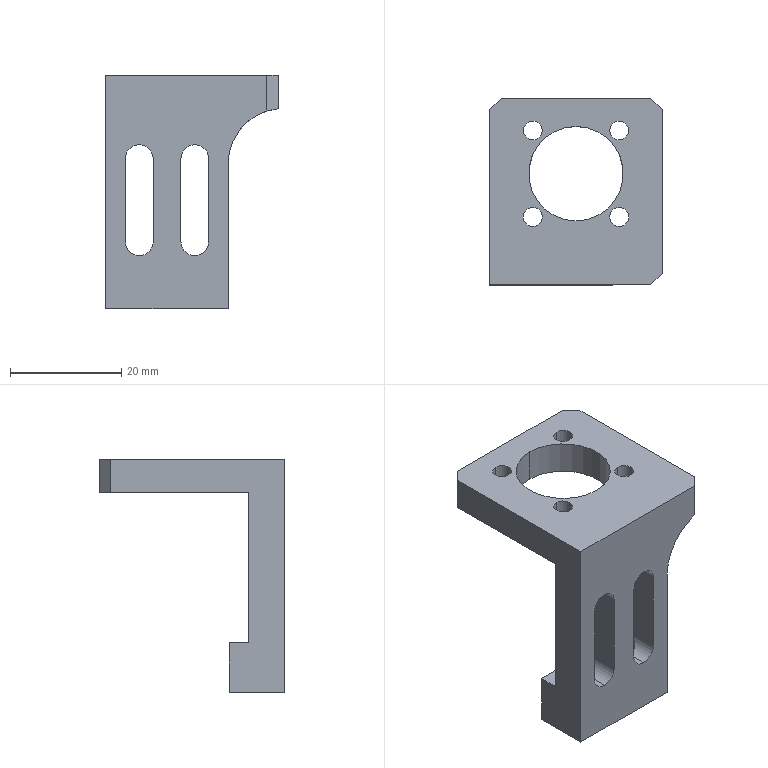NC program | NX | posted with a generic post | part box 31 x 33.478 x 42 mm
Whole program:
N10 G17 G21 G94 G90
(FLOOR_WALL_1 , TOOL : D10)
N12 T15 M6
N14 G54
N16 G17 G0 G90 X22.509 Y-28.409 B0. C0. S9500 M3
N18 G43 Z30. H15
N20 Z-10.428
N22 G94 G1 Z-13.428 F1000.
N24 X21.463 Y-26.597
N26 G3 X20.597 Y-26.097 R1.
N28 G1 X-11.597 F3000.
N30 Y-25.597
N32 X20.597
N34 Y-25.097
N36 X-11.597
N38 Y-24.597
N40 X20.597
N42 Y-24.097
N44 X-11.597
N46 Y-23.597
N48 X20.597
N50 Y-23.097
N52 X-11.597
N54 Y-22.597
N56 X20.597
N58 Y-22.097
N60 X-11.597
N62 Y-21.597
N64 X20.597
N66 Y-21.097
N68 X-11.597
N70 Y-20.597
N72 X20.597
N74 Y-20.097
N76 X-11.597
N78 Y-19.598
N80 X20.597
N82 Y-19.098
N84 X-11.597
N86 Y-18.598
N88 X20.597
N90 Y-18.098
N92 X-11.597
N94 Y-17.598
N96 X20.597
N98 Y-17.098
N100 X-11.597
N102 Y-16.598
N104 X20.597
N106 Y-16.098
N108 X-11.597
N110 Y-15.598
N112 X20.597
N114 Y-15.098
N116 X-11.597
N118 Y-14.598
N120 X20.597
N122 Y-14.098
N124 X-11.597
N126 Y-13.598
N128 X20.597
N130 Y-13.098
N132 X-11.597
N134 Y-12.598
N136 X20.597
N138 Y-12.098
N140 X-11.597
N142 Y-11.598
N144 X20.597
N146 Y-11.098
N148 X-11.597
N150 Y-10.598
N152 X20.597
N154 Y-10.098
N156 X-11.597
N158 Y-9.598
N160 X20.597
N162 Y-9.098
N164 X-11.597
N166 Y-8.598
N168 X20.597
N170 Y-8.099
N172 X-11.597
N174 Y-7.599
N176 X20.597
N178 Y-7.099
N180 X-11.597
N182 Y-6.599
N184 X20.597
N186 Y-6.099
N188 X-11.597
N190 Y-5.599
N192 X20.597
N194 Y-5.099
N196 X-11.597
N198 Y-4.599
N200 X20.597
N202 Y-4.099
N204 X-11.597
N206 Y-3.599
N208 X20.597
N210 Y-3.099
N212 X-11.597
N214 Y-2.599
N216 X20.597
N218 Y-2.099
N220 X-11.597
N222 Y-1.599
N224 X20.597
N226 Y-1.099
N228 X-11.597
N230 Y-0.599
N232 X20.597
N234 Y-0.099
N236 X-11.597
N238 Y0.401
N240 X20.597
N242 Y0.901
N244 X-11.597
N246 Y1.401
N248 X20.597
N250 Y1.901
N252 X-11.597
N254 Y2.401
N256 X20.597
N258 Y2.901
N260 X-11.597
N262 Y3.401
N264 X20.597
N266 Y3.9
N268 X-11.597
N270 Y4.4
N272 X20.597
N274 Y4.9
N276 X-11.597
N278 X-11.61 Y5.4
N280 X20.597
N282 Y5.9
N284 X-11.671
N286 X-11.787 Y6.4
N288 X20.597
N290 Y6.9
N292 X-11.959
N294 X-12.197 Y7.4
N296 X20.597
N298 Y7.9
N300 X-12.51
N302 X-12.92 Y8.4
N304 X20.597
N306 Y8.9
N308 X-13.464
N310 X-14.238 Y9.4
N312 X20.597
N314 Y9.9
N316 X-15.598
N318 G3 X-16.464 Y9.4 R1.
N320 G1 X-17.908 Y6.9
N322 Z-10.428
N324 G0 Z-0.478
N326 X22.509 Y-28.409
N328 Z-20.378
N330 G1 Z-23.378 F1000.
N332 X21.463 Y-26.597
N334 G3 X20.597 Y-26.097 R1.
N336 G1 X-11.597 F3000.
N338 Y-25.597
N340 X20.597
N342 Y-25.097
N344 X-11.597
N346 Y-24.597
N348 X20.597
N350 Y-24.097
N352 X-11.597
N354 Y-23.597
N356 X20.597
N358 Y-23.097
N360 X-11.597
N362 Y-22.597
N364 X20.597
N366 Y-22.097
N368 X-11.597
N370 Y-21.597
N372 X20.597
N374 Y-21.097
N376 X-11.597
N378 Y-20.597
N380 X20.597
N382 Y-20.097
N384 X-11.597
N386 Y-19.598
N388 X20.597
N390 Y-19.098
N392 X-11.597
N394 Y-18.598
N396 X20.597
N398 Y-18.098
N400 X-11.597
N402 Y-17.598
N404 X20.597
N406 Y-17.098
N408 X-11.597
N410 Y-16.598
N412 X20.597
N414 Y-16.098
N416 X-11.597
N418 Y-15.598
N420 X20.597
N422 Y-15.098
N424 X-11.597
N426 Y-14.598
N428 X20.597
N430 Y-14.098
N432 X-11.597
N434 Y-13.598
N436 X20.597
N438 Y-13.098
N440 X-11.597
N442 Y-12.598
N444 X20.597
N446 Y-12.098
N448 X-11.597
N450 Y-11.598
N452 X20.597
N454 Y-11.098
N456 X-11.597
N458 Y-10.598
N460 X20.597
N462 Y-10.098
N464 X-11.597
N466 Y-9.598
N468 X20.597
N470 Y-9.098
N472 X-11.597
N474 Y-8.598
N476 X20.597
N478 Y-8.099
N480 X-11.597
N482 Y-7.599
N484 X20.597
N486 Y-7.099
N488 X-11.597
N490 Y-6.599
N492 X20.597
N494 Y-6.099
N496 X-11.597
N498 Y-5.599
N500 X20.597
N502 Y-5.099
N504 X-11.597
N506 Y-4.599
N508 X20.597
N510 Y-4.099
N512 X-11.597
N514 Y-3.599
N516 X20.597
N518 Y-3.099
N520 X-11.597
N522 Y-2.599
N524 X20.597
N526 Y-2.099
N528 X-11.597
N530 Y-1.599
N532 X20.597
N534 Y-1.099
N536 X-11.597
N538 Y-0.599
N540 X20.597
N542 Y-0.099
N544 X-11.597
N546 Y0.401
N548 X20.597
N550 Y0.901
N552 X-11.597
N554 Y1.401
N556 X20.597
N558 Y1.901
N560 X-11.597
N562 Y2.401
N564 X20.597
N566 Y2.901
N568 X-11.597
N570 Y3.401
N572 X20.597
N574 Y3.9
N576 X-11.597
N578 Y4.4
N580 X20.597
N582 Y4.9
N584 X-11.597
N586 X-11.61 Y5.4
N588 X20.597
N590 Y5.9
N592 X-11.671
N594 X-11.787 Y6.4
N596 X20.597
N598 Y6.9
N600 X-11.959
N602 X-12.197 Y7.4
N604 X20.597
N606 Y7.9
N608 X-12.51
N610 X-12.92 Y8.4
N612 X20.597
N614 Y8.9
N616 X-13.464
N618 X-14.238 Y9.4
N620 X20.597
N622 Y9.9
N624 X-15.598
N626 G3 X-16.464 Y9.4 R1.
N628 G1 X-17.908 Y6.9
N630 Z-20.378
N632 G0 Z30.
(FLOOR_WALL_1_COPY , TOOL : D10)
N634 X23.6 Y-9.211
N636 Z-23.878
N638 G1 Z-26.878 F1000.
N640 X21.097 Y-7.766
N642 G2 X20.597 Y-6.9 R1.
N644 G1 Y9.9 F3000.
N646 X20.098
N648 Y-6.9
N650 X19.598
N652 Y9.9
N654 X19.099
N656 Y-6.9
N658 X18.6
N660 Y9.9
N662 X18.1
N664 Y-6.9
N666 X17.601
N668 Y9.9
N670 X17.102
N672 Y-6.9
N674 X16.602
N676 Y9.9
N678 X16.103
N680 Y-6.9
N682 X15.604
N684 Y9.9
N686 X15.104
N688 Y-6.9
N690 X14.605
N692 Y9.9
N694 X14.105
N696 Y-6.9
N698 X13.606
N700 Y9.9
N702 X13.107
N704 Y-6.9
N706 X12.607
N708 Y9.9
N710 X12.108
N712 Y-6.9
N714 X11.609
N716 Y9.9
N718 X11.109
N720 Y-6.9
N722 X10.61
N724 Y9.9
N726 X10.111
N728 Y-6.9
N730 X9.611
N732 Y9.9
N734 X9.112
N736 Y-6.9
N738 X8.613
N740 Y9.9
N742 X8.113
N744 Y-6.9
N746 X7.614
N748 Y9.9
N750 X7.115
N752 Y-6.9
N754 X6.615
N756 Y9.9
N758 X6.116
N760 Y-6.9
N762 X5.617
N764 Y9.9
N766 X5.117
N768 Y-6.9
N770 X4.618
N772 Y9.9
N774 X4.118
N776 Y-6.9
N778 X3.619
N780 Y9.9
N782 X3.12
N784 Y-6.9
N786 X2.62
N788 Y9.9
N790 X2.121
N792 Y-6.9
N794 X1.622
N796 Y9.9
N798 X1.122
N800 Y-6.9
N802 X0.623
N804 Y9.9
N806 X0.124
N808 Y-6.9
N810 X-0.376
N812 Y9.9
N814 X-0.875
N816 Y-6.9
N818 X-1.374
N820 Y9.9
N822 X-1.874
N824 Y-6.9
N826 X-2.373
N828 Y9.9
N830 X-2.872
N832 Y-6.9
N834 X-3.372
N836 Y9.9
N838 X-3.871
N840 Y-6.9
N842 X-4.37
N844 Y9.9
N846 X-4.87
N848 Y-6.9
N850 X-5.369
N852 Y9.9
N854 X-5.868
N856 Y-6.9
N858 X-6.368
N860 Y9.9
N862 X-6.867
N864 Y9.896
N866 X-7.367
N868 Y9.9
N870 X-7.866
N872 Y9.896
N874 X-8.365
N876 Y9.9
N878 X-8.865
N880 Y9.896
N882 X-9.364
N884 Y9.9
N886 X-9.863
N888 Y9.896
N890 X-10.363
N892 Y9.9
N894 X-10.862
N896 Y9.896
N898 X-11.361
N900 Y9.9
N902 X-11.861
N904 Y6.636
N906 X-12.36 Y7.677
N908 Y9.9
N910 X-12.859
N912 Y8.334
N914 X-13.359 Y8.815
N916 Y9.9
N918 X-13.858
N920 Y9.18
N922 X-14.357 Y9.46
N924 Y9.9
N926 X-14.857
N928 Y9.67
N930 X-15.356 Y9.818
N932 Y9.9
N934 G2 X-14.708 Y9.139 R1.
N936 G1 X-15.736 Y6.793
N938 Z-23.878
N940 G0 Z30.
N942 M5
(FLOOR_WALL_1_COPY_COPY , TOOL : D10JING)
N944 T14 M6
N946 G54
N948 G17 G0 G90 X22.412 Y-4.688 B0. C0. S9500 M3
N950 G43 Z30. H14
N952 Z-20.478
N954 G94 G1 Z-23.478 F1000.
N956 X21.366 Y-6.5
N958 G2 X20.5 Y-7. R1.
N960 G1 X-11.5 F1500.
N962 Y-12.
N964 X20.5
N966 Y-17.
N968 X-11.5
N970 G2 X-12.366 Y-16.5 R1.
N972 G1 X-14.5 Y-12.804
N974 Z-20.478
N976 G0 Z30.
N978 X23.6 Y-5.897
N980 Z-23.978
N982 G1 Z-26.978 F1000.
N984 X19.634
N986 G3 X20.5 Y-6.397 R1.
N988 G1 X-11.5 F1500.
N990 Y-2.448
N992 X20.5
N994 Y1.501
N996 X-11.5
N998 X-11.516 Y5.451
N1000 X20.5
N1002 Y9.4
N1004 X-14.035
N1006 G3 X-14.901 Y8.9 R1.
N1008 G1 X-16.055 Y6.9
N1010 Z-23.978
N1012 G0 Z-23.878
N1014 X-14.5 Y-2.704
N1016 Z-23.978
N1018 G1 Z-26.978 F1000.
N1020 X-12.366 Y-6.4
N1022 G3 X-11.5 Y-6.9 R1.
N1024 G1 X20.5 F1500.
N1026 G3 X21.366 Y-6.4 R1.
N1028 G1 X23.5 Y-2.704
N1030 Z-23.978
N1032 G0 Z-23.878
N1034 Y5.704
N1036 Z-23.978
N1038 G1 Z-26.978 F1000.
N1040 X21.366 Y9.4
N1042 G3 X20.5 Y9.9 R1.
N1044 G1 X-15.166 F1500.
N1046 G3 X-16.032 Y9.4 R1.
N1048 G1 X-17.475 Y6.9
N1050 Z-23.978
N1052 G0 Z30.
(FLOOR_WALL_1_COPY_COPY_COPY , TOOL : D10JING)
N1054 X22.809 Y7.
N1056 Z-8.978
N1058 G1 Z-11.978 F1000.
N1060 X21.366 Y9.5
N1062 G3 X20.5 Y10. R1.
N1064 G1 X-15.606 F1500.
N1066 G3 X-16.472 Y9.5 R1.
N1068 G1 X-17.915 Y7.
N1070 Z-8.978
N1072 G0 Z6.022
N1074 X-12.366 Y-6.5
N1076 Z-8.978
N1078 G1 Z-11.978 F1000.
N1080 G3 X-11.5 Y-7. R1.
N1082 G1 X20.5 F1500.
N1084 G3 X21.366 Y-6.5 R1.
N1086 G1 Z-8.978
N1088 G0 Z6.022
N1090 X22.809 Y7.
N1092 Z-23.978
N1094 G1 Z-26.978 F1000.
N1096 X21.366 Y9.5
N1098 G3 X20.5 Y10. R1.
N1100 G1 X-15.606 F1500.
N1102 G3 X-16.472 Y9.5 R1.
N1104 G1 X-17.915 Y7.
N1106 Z-23.978
N1108 G0 Z-8.978
N1110 X-13.809 Y-4.
N1112 Z-23.978
N1114 G1 Z-26.978 F1000.
N1116 X-12.366 Y-6.5
N1118 G3 X-11.5 Y-7. R1.
N1120 G1 X20.5 F1500.
N1122 G3 X21.366 Y-6.5 R1.
N1124 G1 X22.809 Y-4.
N1126 Z-23.978
N1128 G0 Z30.
N1130 M5
(PLANAR_MILL_COPY_COPY_1_COPY_1 , TOOL : D6A45)
N1132 T01 M6
N1134 G54
N1136 G17 G0 G90 X3.634 Y-10.6 B0. C0. S9500 M3
N1138 G43 Z30. H1
N1140 Z-22.978
N1142 G94 G1 Z-24.478 F1250.
N1144 G3 X4.5 Y-11.1 R1.
N1146 G1 X15.5
N1148 G2 X16.4 Y-12. R0.9
N1150 G1 Y-21.
N1152 G2 X15.5 Y-21.9 R0.9
N1154 G1 X-6.5
N1156 G2 X-7.4 Y-21. R0.9
N1158 G1 Y-12.
N1160 G2 X-6.5 Y-11.1 R0.9
N1162 G1 X4.5
N1164 G3 X5.366 Y-10.6 R1.
N1166 G1 Z-22.978
N1168 G0 Z30.
(PLANAR_MILL_COPY_COPY_1_COPY_1_COPY , TOOL : D6A45)
N1170 X-0.17 Y-7.3
N1172 Z-26.478
N1174 G1 Z-27.978
N1176 X0.234 Y-8.
N1178 G3 X1.1 Y-8.5 R1.
N1180 G1 Y6.
N1182 G3 X-0.5 Y7.6 R1.6
N1184 X-2.1 Y6. R1.6
N1186 G1 Y-8.5
N1188 G3 X-1.234 Y-8. R1.
N1190 G1 X-0.83 Y-7.3
N1192 Z-26.478
N1194 G0 Z30.
N1196 X-8.813 Y-7.908
N1198 Z-26.478
N1200 G1 Z-27.978
N1202 X-8.365 Y-8.357
N1204 G3 X-7.4 Y-8.618 R1.
N1206 G1 Y5.05
N1208 G3 X-10.081 Y11.5 R9.1
N1210 X-10.947 Y11. R1.
N1212 G1 X-11.351 Y10.3
N1214 Z-26.478
N1216 G0 Z30.
N1218 X17.813 Y10.908
N1220 Z-26.478
N1222 G1 Z-27.978
N1224 X17.365 Y11.357
N1226 G3 X16.4 Y11.618 R1.
N1228 G1 Y-8.618
N1230 G3 X17.365 Y-8.357 R1.
N1232 G1 X17.813 Y-7.908
N1234 Z-26.478
N1236 G0 Z30.
N1238 X9.83 Y-7.3
N1240 Z-26.478
N1242 G1 Z-27.978
N1244 X10.234 Y-8.
N1246 G3 X11.1 Y-8.5 R1.
N1248 G1 Y6.
N1250 G3 X9.5 Y7.6 R1.6
N1252 X7.9 Y6. R1.6
N1254 G1 Y-8.5
N1256 G3 X8.766 Y-8. R1.
N1258 G1 X9.17 Y-7.3
N1260 Z-26.478
N1262 G0 Z30.
N1264 M5
N1266 M2